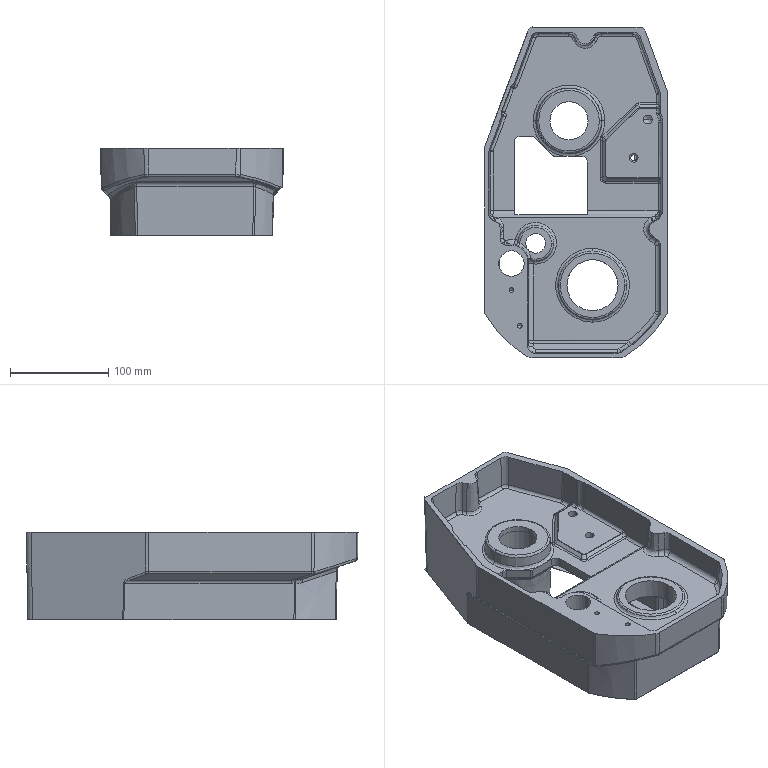Part | SolidWorks | features ICE 8, BaseBody 7, HoleWzd 2 | 1 solid | 615 faces | box 186.612 x 338.668 x 89.052 mm | volume 1423042 mm3 | spline 249 | cylinder 178 | plane 134 | cone 35 | torus 16 | sphere 3 | commonest cylinder face diameters 6 x42 10 x38 12 x19 2 x11 4 x11 14 x5